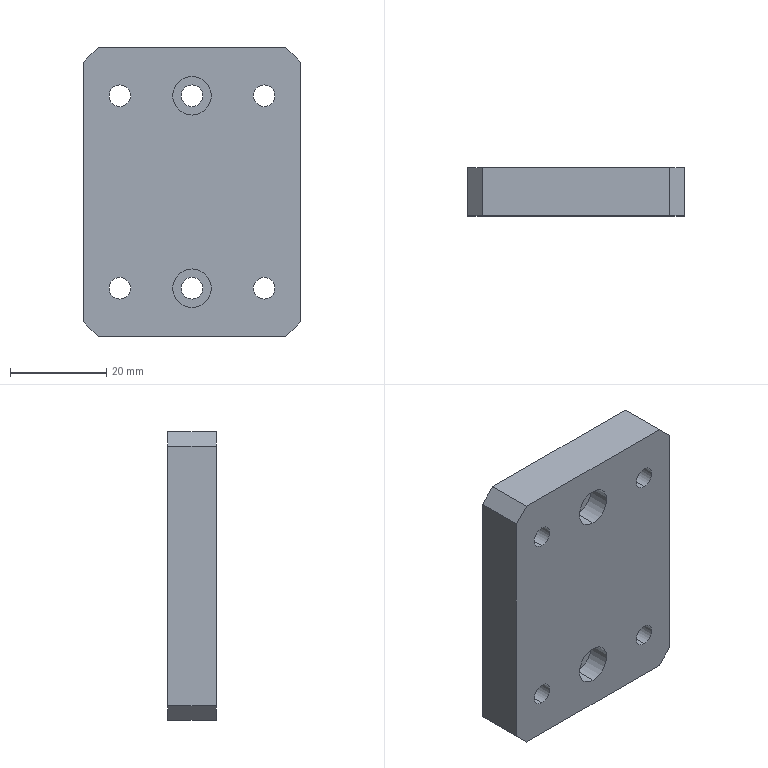Part | STEP file | Camera bracket base plate | 1 solid | 28 faces | box 45 x 10 x 60 mm | volume 25550 mm3 | cylinder 16 | plane 12 | commonest cylinder face diameters 4.5 x12 8 x4